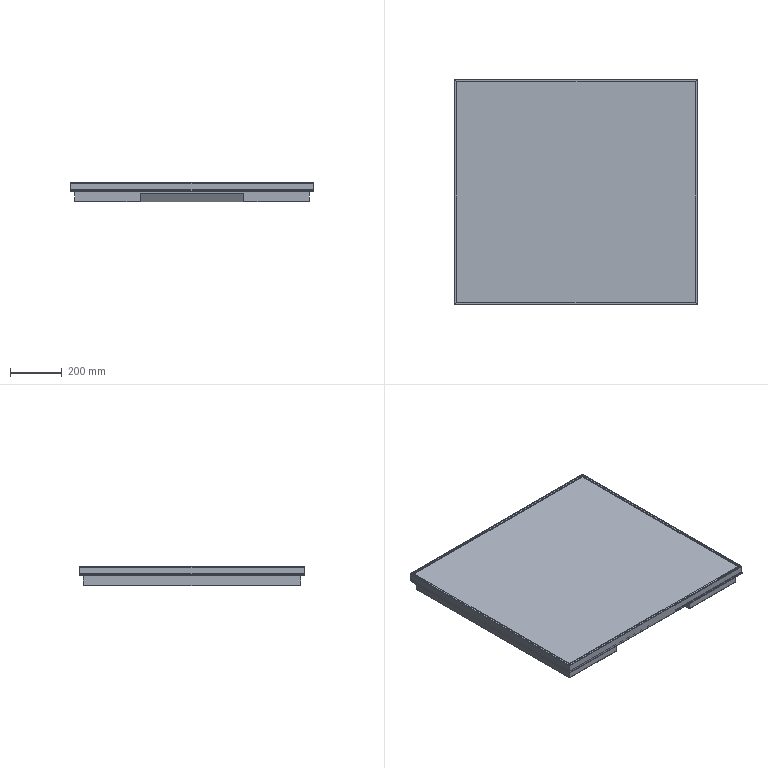Part | 7 solids | 264 faces | box 940 x 870 x 75 mm | volume 3854341 mm3 | plane 176 | cylinder 76 | spline 12 | commonest cylinder face diameters 7 x30 11 x16 0.4 x9 2.4 x9 2 x6 1 x4